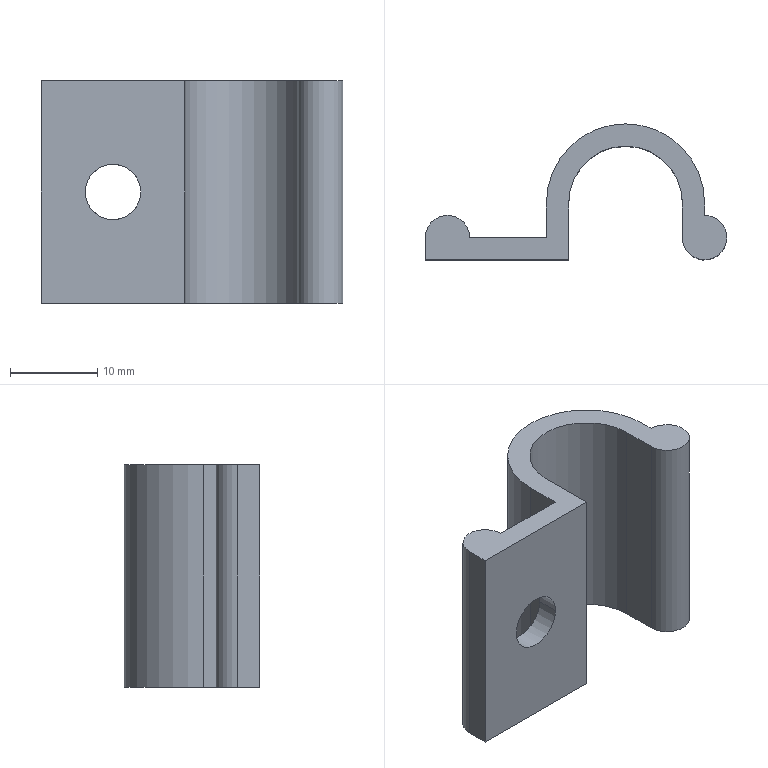Part | STEP file | tubing_clipV11_6.01 - 12.70mm Dia | 1 solid | 15 faces | box 34.48 x 15.54 x 25.4 mm | volume 3707 mm3 | plane 9 | cylinder 6 | commonest cylinder face diameters 5.08 x2 6.35 x2 13 x1 18.08 x1
STEP:
#1=CARTESIAN_POINT('',(0.,0.,0.));
#2=DIRECTION('',(0.,0.,1.));
#3=DIRECTION('',(1.,0.,0.));
#4=AXIS2_PLACEMENT_3D('',#1,#2,#3);
#5=CARTESIAN_POINT('',(-17.82,-3.96,-0.5884));
#6=VERTEX_POINT('',#5);
#7=CARTESIAN_POINT('',(-11.525,-3.96,0.));
#8=VERTEX_POINT('',#7);
#9=CARTESIAN_POINT('',(-14.7,-3.96,0.));
#10=DIRECTION('',(0.,-1.,0.));
#11=DIRECTION('',(1.,0.,0.));
#12=AXIS2_PLACEMENT_3D('',#9,#10,#11);
#13=CIRCLE('',#12,3.175);
#14=CARTESIAN_POINT('',(-14.7,9.04,0.));
#15=DIRECTION('',(0.,-1.,0.));
#16=DIRECTION('',(1.,0.,0.));
#17=AXIS2_PLACEMENT_3D('',#14,#15,#16);
#18=CYLINDRICAL_SURFACE('',#17,3.175);
#19=CARTESIAN_POINT('',(0.,13.));
#20=DIRECTION('',(1.,0.));
#21=VECTOR('',#20,1.);
#22=LINE('',#19,#21);
#23=(GEOMETRIC_REPRESENTATION_CONTEXT(2)PARAMETRIC_REPRESENTATION_CONTEXT()REPRESENTATION_CONTEXT('',''));
#24=DEFINITIONAL_REPRESENTATION('',(#22),#23);
#25=PCURVE('',#18,#24);
#26=CARTESIAN_POINT('',(-17.82,-3.96,12.7));
#27=DIRECTION('',(0.,-1.,0.));
#28=DIRECTION('',(1.,0.,0.));
#29=AXIS2_PLACEMENT_3D('',#26,#27,#28);
#30=PLANE('',#29);
#31=CARTESIAN_POINT('',(3.12,-12.7));
#32=DIRECTION('',(1.,0.));
#33=AXIS2_PLACEMENT_2D('',#31,#32);
#34=CIRCLE('',#33,3.175);
#35=(GEOMETRIC_REPRESENTATION_CONTEXT(2)PARAMETRIC_REPRESENTATION_CONTEXT()REPRESENTATION_CONTEXT('',''));
#36=DEFINITIONAL_REPRESENTATION('',(#34),#35);
#37=PCURVE('',#30,#36);
#38=SURFACE_CURVE('',#13,(#25,#37),.PCURVE_S1.);
#39=EDGE_CURVE('',#6,#8,#38,.T.);
#40=ORIENTED_EDGE('',*,*,#39,.T.);
#41=CARTESIAN_POINT('',(-11.525,-6.5,0.));
#42=VERTEX_POINT('',#41);
#43=CARTESIAN_POINT('',(-11.525,9.04,0.));
#44=DIRECTION('',(0.,-1.,0.));
#45=VECTOR('',#44,1.);
#46=LINE('',#43,#45);
#47=CARTESIAN_POINT('',(6.283,0.));
#48=DIRECTION('',(0.,1.));
#49=VECTOR('',#48,1.);
#50=LINE('',#47,#49);
#51=(GEOMETRIC_REPRESENTATION_CONTEXT(2)PARAMETRIC_REPRESENTATION_CONTEXT()REPRESENTATION_CONTEXT('',''));
#52=DEFINITIONAL_REPRESENTATION('',(#50),#51);
#53=PCURVE('',#18,#52);
#54=CARTESIAN_POINT('',(-14.7,9.04,0.));
#55=DIRECTION('',(0.,-1.,0.));
#56=DIRECTION('',(1.,0.,0.));
#57=AXIS2_PLACEMENT_3D('',#54,#55,#56);
#58=CYLINDRICAL_SURFACE('',#57,3.175);
#59=CARTESIAN_POINT('',(0.,0.));
#60=DIRECTION('',(0.,1.));
#61=VECTOR('',#60,1.);
#62=LINE('',#59,#61);
#63=(GEOMETRIC_REPRESENTATION_CONTEXT(2)PARAMETRIC_REPRESENTATION_CONTEXT()REPRESENTATION_CONTEXT('',''));
#64=DEFINITIONAL_REPRESENTATION('',(#62),#63);
#65=PCURVE('',#58,#64);
#66=SURFACE_CURVE('',#46,(#53,#65),.PCURVE_S1.);
#67=EDGE_CURVE('',#8,#42,#66,.T.);
#68=ORIENTED_EDGE('',*,*,#67,.T.);
#69=CARTESIAN_POINT('',(-17.875,-6.5,0.));
#70=VERTEX_POINT('',#69);
#71=CARTESIAN_POINT('',(-14.7,-6.5,0.));
#72=DIRECTION('',(0.,-1.,0.));
#73=DIRECTION('',(1.,0.,0.));
#74=AXIS2_PLACEMENT_3D('',#71,#72,#73);
#75=CIRCLE('',#74,3.175);
#76=CARTESIAN_POINT('',(0.,15.54));
#77=DIRECTION('',(1.,0.));
#78=VECTOR('',#77,1.);
#79=LINE('',#76,#78);
#80=(GEOMETRIC_REPRESENTATION_CONTEXT(2)PARAMETRIC_REPRESENTATION_CONTEXT()REPRESENTATION_CONTEXT('',''));
#81=DEFINITIONAL_REPRESENTATION('',(#79),#80);
#82=PCURVE('',#18,#81);
#83=CARTESIAN_POINT('',(-6.5,-6.5,12.7));
#84=DIRECTION('',(0.,1.,0.));
#85=DIRECTION('',(-1.,0.,0.));
#86=AXIS2_PLACEMENT_3D('',#83,#84,#85);
#87=PLANE('',#86);
#88=CARTESIAN_POINT('',(5.025,-12.7));
#89=CARTESIAN_POINT('',(5.025,-7.201));
#90=CARTESIAN_POINT('',(9.787,-9.95));
#91=CARTESIAN_POINT('',(14.55,-12.7));
#92=CARTESIAN_POINT('',(9.787,-15.45));
#93=CARTESIAN_POINT('',(5.025,-18.199));
#94=CARTESIAN_POINT('',(5.025,-12.7));
#95=(BOUNDED_CURVE()B_SPLINE_CURVE(2,(#88,#89,#90,#91,#92,#93,#94),.UNSPECIFIED.,.T.,.F.)B_SPLINE_CURVE_WITH_KNOTS((1,2,2,2,2,1),(-2.094,0.,2.094,4.189,6.283,8.378),.UNSPECIFIED.)CURVE()GEOMETRIC_REPRESENTATION_ITEM()RATIONAL_B_SPLINE_CURVE((1.,0.5,1.,0.5,1.,0.5,1.))REPRESENTATION_ITEM(''));
#96=(GEOMETRIC_REPRESENTATION_CONTEXT(2)PARAMETRIC_REPRESENTATION_CONTEXT()REPRESENTATION_CONTEXT('',''));
#97=DEFINITIONAL_REPRESENTATION('',(#95),#96);
#98=PCURVE('',#87,#97);
#99=SURFACE_CURVE('',#75,(#82,#98),.PCURVE_S1.);
#100=EDGE_CURVE('',#70,#42,#99,.T.);
#101=ORIENTED_EDGE('',*,*,#100,.F.);
#102=CARTESIAN_POINT('',(-17.875,-3.434,0.));
#103=VERTEX_POINT('',#102);
#104=CARTESIAN_POINT('',(-17.875,9.04,0.));
#105=DIRECTION('',(0.,-1.,0.));
#106=VECTOR('',#105,1.);
#107=LINE('',#104,#106);
#108=CARTESIAN_POINT('',(3.142,0.));
#109=DIRECTION('',(0.,1.));
#110=VECTOR('',#109,1.);
#111=LINE('',#108,#110);
#112=(GEOMETRIC_REPRESENTATION_CONTEXT(2)PARAMETRIC_REPRESENTATION_CONTEXT()REPRESENTATION_CONTEXT('',''));
#113=DEFINITIONAL_REPRESENTATION('',(#111),#112);
#114=PCURVE('',#18,#113);
#115=CARTESIAN_POINT('',(3.142,0.));
#116=DIRECTION('',(0.,1.));
#117=VECTOR('',#116,1.);
#118=LINE('',#115,#117);
#119=(GEOMETRIC_REPRESENTATION_CONTEXT(2)PARAMETRIC_REPRESENTATION_CONTEXT()REPRESENTATION_CONTEXT('',''));
#120=DEFINITIONAL_REPRESENTATION('',(#118),#119);
#121=PCURVE('',#58,#120);
#122=SURFACE_CURVE('',#107,(#114,#121),.PCURVE_S1.);
#123=EDGE_CURVE('',#103,#70,#122,.T.);
#124=ORIENTED_EDGE('',*,*,#123,.F.);
#125=CARTESIAN_POINT('',(-17.875,-3.434,0.));
#126=CARTESIAN_POINT('',(-17.875,-3.434,-0.1473));
#127=CARTESIAN_POINT('',(-17.864,-3.482,-0.2926));
#128=CARTESIAN_POINT('',(-17.835,-3.671,-0.5171));
#129=CARTESIAN_POINT('',(-17.82,-3.812,-0.5884));
#130=CARTESIAN_POINT('',(-17.82,-3.96,-0.5884));
#131=B_SPLINE_CURVE_WITH_KNOTS('',3,(#125,#126,#127,#128,#129,#130),.UNSPECIFIED.,.F.,.F.,(4,2,4),(0.0008744,0.001312,0.00175),.UNSPECIFIED.);
#132=CARTESIAN_POINT('',(3.142,12.474));
#133=CARTESIAN_POINT('',(3.146,12.474));
#134=CARTESIAN_POINT('',(3.154,12.475));
#135=CARTESIAN_POINT('',(3.167,12.479));
#136=CARTESIAN_POINT('',(3.179,12.485));
#137=CARTESIAN_POINT('',(3.192,12.493));
#138=CARTESIAN_POINT('',(3.204,12.503));
#139=CARTESIAN_POINT('',(3.215,12.516));
#140=CARTESIAN_POINT('',(3.227,12.532));
#141=CARTESIAN_POINT('',(3.238,12.549));
#142=CARTESIAN_POINT('',(3.249,12.569));
#143=CARTESIAN_POINT('',(3.26,12.592));
#144=CARTESIAN_POINT('',(3.27,12.616));
#145=CARTESIAN_POINT('',(3.279,12.643));
#146=CARTESIAN_POINT('',(3.288,12.672));
#147=CARTESIAN_POINT('',(3.296,12.703));
#148=CARTESIAN_POINT('',(3.303,12.736));
#149=CARTESIAN_POINT('',(3.309,12.77));
#150=CARTESIAN_POINT('',(3.315,12.806));
#151=CARTESIAN_POINT('',(3.32,12.843));
#152=CARTESIAN_POINT('',(3.323,12.881));
#153=CARTESIAN_POINT('',(3.326,12.92));
#154=CARTESIAN_POINT('',(3.328,12.96));
#155=CARTESIAN_POINT('',(3.328,12.987));
#156=CARTESIAN_POINT('',(3.328,13.));
#157=B_SPLINE_CURVE_WITH_KNOTS('',3,(#132,#133,#134,#135,#136,#137,#138,#139,#140,#141,#142,#143,#144,#145,#146,#147,#148,#149,#150,#151,#152,#153,#154,#155,#156),.UNSPECIFIED.,.F.,.F.,(4,1,1,1,1,1,1,1,1,1,1,1,1,1,1,1,1,1,1,1,1,1,4),(0.0008744,0.0009142,0.000954,0.0009938,0.001034,0.001073,0.001113,0.001153,0.001193,0.001233,0.001272,0.001312,0.001352,0.001392,0.001432,0.001471,0.001511,0.001551,0.001591,0.00163,0.00167,0.00171,0.00175),.QUASI_UNIFORM_KNOTS.);
#158=(GEOMETRIC_REPRESENTATION_CONTEXT(2)PARAMETRIC_REPRESENTATION_CONTEXT()REPRESENTATION_CONTEXT('',''));
#159=DEFINITIONAL_REPRESENTATION('',(#157),#158);
#160=PCURVE('',#18,#159);
#161=CARTESIAN_POINT('',(-20.36,-3.96,12.7));
#162=DIRECTION('',(0.,0.,-1.));
#163=DIRECTION('',(-1.,0.,0.));
#164=AXIS2_PLACEMENT_3D('',#161,#162,#163);
#165=CYLINDRICAL_SURFACE('',#164,2.54);
#166=CARTESIAN_POINT('',(2.933,12.7));
#167=CARTESIAN_POINT('',(2.933,12.713));
#168=CARTESIAN_POINT('',(2.933,12.74));
#169=CARTESIAN_POINT('',(2.935,12.78));
#170=CARTESIAN_POINT('',(2.937,12.82));
#171=CARTESIAN_POINT('',(2.941,12.859));
#172=CARTESIAN_POINT('',(2.945,12.897));
#173=CARTESIAN_POINT('',(2.95,12.934));
#174=CARTESIAN_POINT('',(2.956,12.971));
#175=CARTESIAN_POINT('',(2.963,13.006));
#176=CARTESIAN_POINT('',(2.971,13.041));
#177=CARTESIAN_POINT('',(2.98,13.074));
#178=CARTESIAN_POINT('',(2.99,13.105));
#179=CARTESIAN_POINT('',(3.001,13.135));
#180=CARTESIAN_POINT('',(3.012,13.162));
#181=CARTESIAN_POINT('',(3.024,13.187));
#182=CARTESIAN_POINT('',(3.037,13.21));
#183=CARTESIAN_POINT('',(3.051,13.23));
#184=CARTESIAN_POINT('',(3.065,13.248));
#185=CARTESIAN_POINT('',(3.08,13.262));
#186=CARTESIAN_POINT('',(3.095,13.274));
#187=CARTESIAN_POINT('',(3.11,13.282));
#188=CARTESIAN_POINT('',(3.126,13.287));
#189=CARTESIAN_POINT('',(3.136,13.288));
#190=CARTESIAN_POINT('',(3.142,13.288));
#191=B_SPLINE_CURVE_WITH_KNOTS('',3,(#166,#167,#168,#169,#170,#171,#172,#173,#174,#175,#176,#177,#178,#179,#180,#181,#182,#183,#184,#185,#186,#187,#188,#189,#190),.UNSPECIFIED.,.F.,.F.,(4,1,1,1,1,1,1,1,1,1,1,1,1,1,1,1,1,1,1,1,1,1,4),(0.0008744,0.0009142,0.000954,0.0009938,0.001034,0.001073,0.001113,0.001153,0.001193,0.001233,0.001272,0.001312,0.001352,0.001392,0.001432,0.001471,0.001511,0.001551,0.001591,0.00163,0.00167,0.00171,0.00175),.QUASI_UNIFORM_KNOTS.);
#192=(GEOMETRIC_REPRESENTATION_CONTEXT(2)PARAMETRIC_REPRESENTATION_CONTEXT()REPRESENTATION_CONTEXT('',''));
#193=DEFINITIONAL_REPRESENTATION('',(#191),#192);
#194=PCURVE('',#165,#193);
#195=SURFACE_CURVE('',#131,(#160,#194),.PCURVE_S1.);
#196=EDGE_CURVE('',#103,#6,#195,.T.);
#197=ORIENTED_EDGE('',*,*,#196,.T.);
#198=EDGE_LOOP('',(#40,#68,#101,#124,#197));
#199=FACE_BOUND('',#198,.F.);
#200=ADVANCED_FACE('',(#199),#18,.F.);
#201=CARTESIAN_POINT('',(-14.7,-6.5,0.));
#202=DIRECTION('',(0.,-1.,0.));
#203=DIRECTION('',(1.,0.,0.));
#204=AXIS2_PLACEMENT_3D('',#201,#202,#203);
#205=CIRCLE('',#204,3.175);
#206=CARTESIAN_POINT('',(5.025,-12.7));
#207=CARTESIAN_POINT('',(5.025,-7.201));
#208=CARTESIAN_POINT('',(9.787,-9.95));
#209=CARTESIAN_POINT('',(14.55,-12.7));
#210=CARTESIAN_POINT('',(9.787,-15.45));
#211=CARTESIAN_POINT('',(5.025,-18.199));
#212=CARTESIAN_POINT('',(5.025,-12.7));
#213=(BOUNDED_CURVE()B_SPLINE_CURVE(2,(#206,#207,#208,#209,#210,#211,#212),.UNSPECIFIED.,.T.,.F.)B_SPLINE_CURVE_WITH_KNOTS((1,2,2,2,2,1),(-2.094,0.,2.094,4.189,6.283,8.378),.UNSPECIFIED.)CURVE()GEOMETRIC_REPRESENTATION_ITEM()RATIONAL_B_SPLINE_CURVE((1.,0.5,1.,0.5,1.,0.5,1.))REPRESENTATION_ITEM(''));
#214=(GEOMETRIC_REPRESENTATION_CONTEXT(2)PARAMETRIC_REPRESENTATION_CONTEXT()REPRESENTATION_CONTEXT('',''));
#215=DEFINITIONAL_REPRESENTATION('',(#213),#214);
#216=PCURVE('',#87,#215);
#217=CARTESIAN_POINT('',(0.,15.54));
#218=DIRECTION('',(1.,0.));
#219=VECTOR('',#218,1.);
#220=LINE('',#217,#219);
#221=(GEOMETRIC_REPRESENTATION_CONTEXT(2)PARAMETRIC_REPRESENTATION_CONTEXT()REPRESENTATION_CONTEXT('',''));
#222=DEFINITIONAL_REPRESENTATION('',(#220),#221);
#223=PCURVE('',#58,#222);
#224=SURFACE_CURVE('',#205,(#216,#223),.PCURVE_S1.);
#225=EDGE_CURVE('',#42,#70,#224,.T.);
#226=ORIENTED_EDGE('',*,*,#225,.F.);
#227=ORIENTED_EDGE('',*,*,#100,.F.);
#228=EDGE_LOOP('',(#226,#227));
#229=FACE_BOUND('',#228,.T.);
#230=CARTESIAN_POINT('',(-22.9,-6.5,-12.7));
#231=VERTEX_POINT('',#230);
#232=CARTESIAN_POINT('',(-6.5,-6.5,-12.7));
#233=VERTEX_POINT('',#232);
#234=CARTESIAN_POINT('',(-6.5,-6.5,-12.7));
#235=DIRECTION('',(1.,0.,0.));
#236=VECTOR('',#235,1.);
#237=LINE('',#234,#236);
#238=CARTESIAN_POINT('',(0.,-25.4));
#239=DIRECTION('',(-1.,0.));
#240=VECTOR('',#239,1.);
#241=LINE('',#238,#240);
#242=(GEOMETRIC_REPRESENTATION_CONTEXT(2)PARAMETRIC_REPRESENTATION_CONTEXT()REPRESENTATION_CONTEXT('',''));
#243=DEFINITIONAL_REPRESENTATION('',(#241),#242);
#244=PCURVE('',#87,#243);
#245=CARTESIAN_POINT('',(-20.36,-3.96,-12.7));
#246=DIRECTION('',(0.,0.,1.));
#247=DIRECTION('',(1.,0.,0.));
#248=AXIS2_PLACEMENT_3D('',#245,#246,#247);
#249=PLANE('',#248);
#250=CARTESIAN_POINT('',(13.86,-2.54));
#251=DIRECTION('',(1.,0.));
#252=VECTOR('',#251,1.);
#253=LINE('',#250,#252);
#254=(GEOMETRIC_REPRESENTATION_CONTEXT(2)PARAMETRIC_REPRESENTATION_CONTEXT()REPRESENTATION_CONTEXT('',''));
#255=DEFINITIONAL_REPRESENTATION('',(#253),#254);
#256=PCURVE('',#249,#255);
#257=SURFACE_CURVE('',#237,(#244,#256),.PCURVE_S1.);
#258=EDGE_CURVE('',#231,#233,#257,.T.);
#259=ORIENTED_EDGE('',*,*,#258,.T.);
#260=CARTESIAN_POINT('',(-6.5,-6.5,12.7));
#261=VERTEX_POINT('',#260);
#262=CARTESIAN_POINT('',(-6.5,-6.5,12.7));
#263=DIRECTION('',(0.,0.,-1.));
#264=VECTOR('',#263,1.);
#265=LINE('',#262,#264);
#266=CARTESIAN_POINT('',(0.,0.));
#267=DIRECTION('',(0.,-1.));
#268=VECTOR('',#267,1.);
#269=LINE('',#266,#268);
#270=(GEOMETRIC_REPRESENTATION_CONTEXT(2)PARAMETRIC_REPRESENTATION_CONTEXT()REPRESENTATION_CONTEXT('',''));
#271=DEFINITIONAL_REPRESENTATION('',(#269),#270);
#272=PCURVE('',#87,#271);
#273=CARTESIAN_POINT('',(-6.5,0.,12.7));
#274=DIRECTION('',(-1.,0.,0.));
#275=DIRECTION('',(0.,-1.,0.));
#276=AXIS2_PLACEMENT_3D('',#273,#274,#275);
#277=PLANE('',#276);
#278=CARTESIAN_POINT('',(6.5,0.));
#279=DIRECTION('',(0.,-1.));
#280=VECTOR('',#279,1.);
#281=LINE('',#278,#280);
#282=(GEOMETRIC_REPRESENTATION_CONTEXT(2)PARAMETRIC_REPRESENTATION_CONTEXT()REPRESENTATION_CONTEXT('',''));
#283=DEFINITIONAL_REPRESENTATION('',(#281),#282);
#284=PCURVE('',#277,#283);
#285=SURFACE_CURVE('',#265,(#272,#284),.PCURVE_S1.);
#286=EDGE_CURVE('',#261,#233,#285,.T.);
#287=ORIENTED_EDGE('',*,*,#286,.F.);
#288=CARTESIAN_POINT('',(-22.9,-6.5,12.7));
#289=VERTEX_POINT('',#288);
#290=CARTESIAN_POINT('',(-6.5,-6.5,12.7));
#291=DIRECTION('',(1.,0.,0.));
#292=VECTOR('',#291,1.);
#293=LINE('',#290,#292);
#294=CARTESIAN_POINT('',(0.,0.));
#295=DIRECTION('',(-1.,0.));
#296=VECTOR('',#295,1.);
#297=LINE('',#294,#296);
#298=(GEOMETRIC_REPRESENTATION_CONTEXT(2)PARAMETRIC_REPRESENTATION_CONTEXT()REPRESENTATION_CONTEXT('',''));
#299=DEFINITIONAL_REPRESENTATION('',(#297),#298);
#300=PCURVE('',#87,#299);
#301=CARTESIAN_POINT('',(-20.36,-3.96,12.7));
#302=DIRECTION('',(0.,0.,1.));
#303=DIRECTION('',(1.,0.,0.));
#304=AXIS2_PLACEMENT_3D('',#301,#302,#303);
#305=PLANE('',#304);
#306=CARTESIAN_POINT('',(13.86,-2.54));
#307=DIRECTION('',(1.,0.));
#308=VECTOR('',#307,1.);
#309=LINE('',#306,#308);
#310=(GEOMETRIC_REPRESENTATION_CONTEXT(2)PARAMETRIC_REPRESENTATION_CONTEXT()REPRESENTATION_CONTEXT('',''));
#311=DEFINITIONAL_REPRESENTATION('',(#309),#310);
#312=PCURVE('',#305,#311);
#313=SURFACE_CURVE('',#293,(#300,#312),.PCURVE_S1.);
#314=EDGE_CURVE('',#289,#261,#313,.T.);
#315=ORIENTED_EDGE('',*,*,#314,.F.);
#316=CARTESIAN_POINT('',(-22.9,-6.5,12.7));
#317=DIRECTION('',(0.,0.,-1.));
#318=VECTOR('',#317,1.);
#319=LINE('',#316,#318);
#320=CARTESIAN_POINT('',(16.4,0.));
#321=DIRECTION('',(0.,-1.));
#322=VECTOR('',#321,1.);
#323=LINE('',#320,#322);
#324=(GEOMETRIC_REPRESENTATION_CONTEXT(2)PARAMETRIC_REPRESENTATION_CONTEXT()REPRESENTATION_CONTEXT('',''));
#325=DEFINITIONAL_REPRESENTATION('',(#323),#324);
#326=PCURVE('',#87,#325);
#327=CARTESIAN_POINT('',(-22.9,-6.5,12.7));
#328=DIRECTION('',(1.,0.,0.));
#329=DIRECTION('',(0.,0.,-1.));
#330=AXIS2_PLACEMENT_3D('',#327,#328,#329);
#331=PLANE('',#330);
#332=CARTESIAN_POINT('',(0.,0.));
#333=DIRECTION('',(1.,0.));
#334=VECTOR('',#333,1.);
#335=LINE('',#332,#334);
#336=(GEOMETRIC_REPRESENTATION_CONTEXT(2)PARAMETRIC_REPRESENTATION_CONTEXT()REPRESENTATION_CONTEXT('',''));
#337=DEFINITIONAL_REPRESENTATION('',(#335),#336);
#338=PCURVE('',#331,#337);
#339=SURFACE_CURVE('',#319,(#326,#338),.PCURVE_S1.);
#340=EDGE_CURVE('',#289,#231,#339,.T.);
#341=ORIENTED_EDGE('',*,*,#340,.T.);
#342=EDGE_LOOP('',(#259,#287,#315,#341));
#343=FACE_BOUND('',#342,.T.);
#344=ADVANCED_FACE('',(#229,#343),#87,.F.);
#345=CARTESIAN_POINT('',(-6.5,0.,-12.7));
#346=VERTEX_POINT('',#345);
#347=CARTESIAN_POINT('',(-6.5,0.,-12.7));
#348=DIRECTION('',(0.,1.,0.));
#349=VECTOR('',#348,1.);
#350=LINE('',#347,#349);
#351=CARTESIAN_POINT('',(0.,-25.4));
#352=DIRECTION('',(-1.,0.));
#353=VECTOR('',#352,1.);
#354=LINE('',#351,#353);
#355=(GEOMETRIC_REPRESENTATION_CONTEXT(2)PARAMETRIC_REPRESENTATION_CONTEXT()REPRESENTATION_CONTEXT('',''));
#356=DEFINITIONAL_REPRESENTATION('',(#354),#355);
#357=PCURVE('',#277,#356);
#358=CARTESIAN_POINT('',(13.86,3.96));
#359=DIRECTION('',(0.,1.));
#360=VECTOR('',#359,1.);
#361=LINE('',#358,#360);
#362=(GEOMETRIC_REPRESENTATION_CONTEXT(2)PARAMETRIC_REPRESENTATION_CONTEXT()REPRESENTATION_CONTEXT('',''));
#363=DEFINITIONAL_REPRESENTATION('',(#361),#362);
#364=PCURVE('',#249,#363);
#365=SURFACE_CURVE('',#350,(#357,#364),.PCURVE_S1.);
#366=EDGE_CURVE('',#233,#346,#365,.T.);
#367=ORIENTED_EDGE('',*,*,#366,.T.);
#368=CARTESIAN_POINT('',(-6.5,0.,12.7));
#369=VERTEX_POINT('',#368);
#370=CARTESIAN_POINT('',(-6.5,0.,12.7));
#371=DIRECTION('',(0.,0.,-1.));
#372=VECTOR('',#371,1.);
#373=LINE('',#370,#372);
#374=CARTESIAN_POINT('',(0.,0.));
#375=DIRECTION('',(0.,-1.));
#376=VECTOR('',#375,1.);
#377=LINE('',#374,#376);
#378=(GEOMETRIC_REPRESENTATION_CONTEXT(2)PARAMETRIC_REPRESENTATION_CONTEXT()REPRESENTATION_CONTEXT('',''));
#379=DEFINITIONAL_REPRESENTATION('',(#377),#378);
#380=PCURVE('',#277,#379);
#381=CARTESIAN_POINT('',(0.,0.,12.7));
#382=DIRECTION('',(0.,0.,-1.));
#383=DIRECTION('',(-1.,0.,0.));
#384=AXIS2_PLACEMENT_3D('',#381,#382,#383);
#385=CYLINDRICAL_SURFACE('',#384,6.5);
#386=CARTESIAN_POINT('',(0.,0.));
#387=DIRECTION('',(0.,1.));
#388=VECTOR('',#387,1.);
#389=LINE('',#386,#388);
#390=(GEOMETRIC_REPRESENTATION_CONTEXT(2)PARAMETRIC_REPRESENTATION_CONTEXT()REPRESENTATION_CONTEXT('',''));
#391=DEFINITIONAL_REPRESENTATION('',(#389),#390);
#392=PCURVE('',#385,#391);
#393=SURFACE_CURVE('',#373,(#380,#392),.PCURVE_S1.);
#394=EDGE_CURVE('',#369,#346,#393,.T.);
#395=ORIENTED_EDGE('',*,*,#394,.F.);
#396=CARTESIAN_POINT('',(-6.5,0.,12.7));
#397=DIRECTION('',(0.,1.,0.));
#398=VECTOR('',#397,1.);
#399=LINE('',#396,#398);
#400=CARTESIAN_POINT('',(0.,0.));
#401=DIRECTION('',(-1.,0.));
#402=VECTOR('',#401,1.);
#403=LINE('',#400,#402);
#404=(GEOMETRIC_REPRESENTATION_CONTEXT(2)PARAMETRIC_REPRESENTATION_CONTEXT()REPRESENTATION_CONTEXT('',''));
#405=DEFINITIONAL_REPRESENTATION('',(#403),#404);
#406=PCURVE('',#277,#405);
#407=CARTESIAN_POINT('',(13.86,3.96));
#408=DIRECTION('',(0.,1.));
#409=VECTOR('',#408,1.);
#410=LINE('',#407,#409);
#411=(GEOMETRIC_REPRESENTATION_CONTEXT(2)PARAMETRIC_REPRESENTATION_CONTEXT()REPRESENTATION_CONTEXT('',''));
#412=DEFINITIONAL_REPRESENTATION('',(#410),#411);
#413=PCURVE('',#305,#412);
#414=SURFACE_CURVE('',#399,(#406,#413),.PCURVE_S1.);
#415=EDGE_CURVE('',#261,#369,#414,.T.);
#416=ORIENTED_EDGE('',*,*,#415,.F.);
#417=ORIENTED_EDGE('',*,*,#286,.T.);
#418=EDGE_LOOP('',(#367,#395,#416,#417));
#419=FACE_BOUND('',#418,.T.);
#420=ADVANCED_FACE('',(#419),#277,.F.);
#421=ORIENTED_EDGE('',*,*,#394,.F.);
#422=CARTESIAN_POINT('',(6.5,0.,12.7));
#423=VERTEX_POINT('',#422);
#424=CARTESIAN_POINT('',(0.,0.,12.7));
#425=DIRECTION('',(0.,0.,-1.));
#426=DIRECTION('',(1.,0.,0.));
#427=AXIS2_PLACEMENT_3D('',#424,#425,#426);
#428=CIRCLE('',#427,6.5);
#429=CARTESIAN_POINT('',(-3.142,0.));
#430=DIRECTION('',(1.,0.));
#431=VECTOR('',#430,1.);
#432=LINE('',#429,#431);
#433=(GEOMETRIC_REPRESENTATION_CONTEXT(2)PARAMETRIC_REPRESENTATION_CONTEXT()REPRESENTATION_CONTEXT('',''));
#434=DEFINITIONAL_REPRESENTATION('',(#432),#433);
#435=PCURVE('',#385,#434);
#436=CARTESIAN_POINT('',(26.86,3.96));
#437=CARTESIAN_POINT('',(26.86,-7.298));
#438=CARTESIAN_POINT('',(17.11,-1.669));
#439=CARTESIAN_POINT('',(7.36,3.96));
#440=CARTESIAN_POINT('',(17.11,9.589));
#441=CARTESIAN_POINT('',(26.86,15.218));
#442=CARTESIAN_POINT('',(26.86,3.96));
#443=(BOUNDED_CURVE()B_SPLINE_CURVE(2,(#436,#437,#438,#439,#440,#441,#442),.UNSPECIFIED.,.T.,.F.)B_SPLINE_CURVE_WITH_KNOTS((1,2,2,2,2,1),(-2.094,0.,2.094,4.189,6.283,8.378),.UNSPECIFIED.)CURVE()GEOMETRIC_REPRESENTATION_ITEM()RATIONAL_B_SPLINE_CURVE((1.,0.5,1.,0.5,1.,0.5,1.))REPRESENTATION_ITEM(''));
#444=(GEOMETRIC_REPRESENTATION_CONTEXT(2)PARAMETRIC_REPRESENTATION_CONTEXT()REPRESENTATION_CONTEXT('',''));
#445=DEFINITIONAL_REPRESENTATION('',(#443),#444);
#446=PCURVE('',#305,#445);
#447=SURFACE_CURVE('',#428,(#435,#446),.PCURVE_S1.);
#448=EDGE_CURVE('',#369,#423,#447,.T.);
#449=ORIENTED_EDGE('',*,*,#448,.T.);
#450=CARTESIAN_POINT('',(6.5,0.,-12.7));
#451=VERTEX_POINT('',#450);
#452=CARTESIAN_POINT('',(6.5,0.,12.7));
#453=DIRECTION('',(0.,0.,-1.));
#454=VECTOR('',#453,1.);
#455=LINE('',#452,#454);
#456=CARTESIAN_POINT('',(3.142,0.));
#457=DIRECTION('',(0.,1.));
#458=VECTOR('',#457,1.);
#459=LINE('',#456,#458);
#460=(GEOMETRIC_REPRESENTATION_CONTEXT(2)PARAMETRIC_REPRESENTATION_CONTEXT()REPRESENTATION_CONTEXT('',''));
#461=DEFINITIONAL_REPRESENTATION('',(#459),#460);
#462=PCURVE('',#385,#461);
#463=CARTESIAN_POINT('',(6.5,0.,12.7));
#464=DIRECTION('',(1.,0.,0.));
#465=DIRECTION('',(0.,1.,0.));
#466=AXIS2_PLACEMENT_3D('',#463,#464,#465);
#467=PLANE('',#466);
#468=CARTESIAN_POINT('',(0.,0.));
#469=DIRECTION('',(0.,-1.));
#470=VECTOR('',#469,1.);
#471=LINE('',#468,#470);
#472=(GEOMETRIC_REPRESENTATION_CONTEXT(2)PARAMETRIC_REPRESENTATION_CONTEXT()REPRESENTATION_CONTEXT('',''));
#473=DEFINITIONAL_REPRESENTATION('',(#471),#472);
#474=PCURVE('',#467,#473);
#475=SURFACE_CURVE('',#455,(#462,#474),.PCURVE_S1.);
#476=EDGE_CURVE('',#423,#451,#475,.T.);
#477=ORIENTED_EDGE('',*,*,#476,.T.);
#478=CARTESIAN_POINT('',(0.,0.,-12.7));
#479=DIRECTION('',(0.,0.,-1.));
#480=DIRECTION('',(1.,0.,0.));
#481=AXIS2_PLACEMENT_3D('',#478,#479,#480);
#482=CIRCLE('',#481,6.5);
#483=CARTESIAN_POINT('',(-3.142,25.4));
#484=DIRECTION('',(1.,0.));
#485=VECTOR('',#484,1.);
#486=LINE('',#483,#485);
#487=(GEOMETRIC_REPRESENTATION_CONTEXT(2)PARAMETRIC_REPRESENTATION_CONTEXT()REPRESENTATION_CONTEXT('',''));
#488=DEFINITIONAL_REPRESENTATION('',(#486),#487);
#489=PCURVE('',#385,#488);
#490=CARTESIAN_POINT('',(26.86,3.96));
#491=CARTESIAN_POINT('',(26.86,-7.298));
#492=CARTESIAN_POINT('',(17.11,-1.669));
#493=CARTESIAN_POINT('',(7.36,3.96));
#494=CARTESIAN_POINT('',(17.11,9.589));
#495=CARTESIAN_POINT('',(26.86,15.218));
#496=CARTESIAN_POINT('',(26.86,3.96));
#497=(BOUNDED_CURVE()B_SPLINE_CURVE(2,(#490,#491,#492,#493,#494,#495,#496),.UNSPECIFIED.,.T.,.F.)B_SPLINE_CURVE_WITH_KNOTS((1,2,2,2,2,1),(-2.094,0.,2.094,4.189,6.283,8.378),.UNSPECIFIED.)CURVE()GEOMETRIC_REPRESENTATION_ITEM()RATIONAL_B_SPLINE_CURVE((1.,0.5,1.,0.5,1.,0.5,1.))REPRESENTATION_ITEM(''));
#498=(GEOMETRIC_REPRESENTATION_CONTEXT(2)PARAMETRIC_REPRESENTATION_CONTEXT()REPRESENTATION_CONTEXT('',''));
#499=DEFINITIONAL_REPRESENTATION('',(#497),#498);
#500=PCURVE('',#249,#499);
#501=SURFACE_CURVE('',#482,(#489,#500),.PCURVE_S1.);
#502=EDGE_CURVE('',#346,#451,#501,.T.);
#503=ORIENTED_EDGE('',*,*,#502,.F.);
#504=EDGE_LOOP('',(#421,#449,#477,#503));
#505=FACE_BOUND('',#504,.F.);
#506=ADVANCED_FACE('',(#505),#385,.F.);
#507=CARTESIAN_POINT('',(6.5,-3.96,-12.7));
#508=VERTEX_POINT('',#507);
#509=CARTESIAN_POINT('',(6.5,0.,-12.7));
#510=DIRECTION('',(0.,-1.,0.));
#511=VECTOR('',#510,1.);
#512=LINE('',#509,#511);
#513=CARTESIAN_POINT('',(0.,-25.4));
#514=DIRECTION('',(-1.,0.));
#515=VECTOR('',#514,1.);
#516=LINE('',#513,#515);
#517=(GEOMETRIC_REPRESENTATION_CONTEXT(2)PARAMETRIC_REPRESENTATION_CONTEXT()REPRESENTATION_CONTEXT('',''));
#518=DEFINITIONAL_REPRESENTATION('',(#516),#517);
#519=PCURVE('',#467,#518);
#520=CARTESIAN_POINT('',(26.86,3.96));
#521=DIRECTION('',(0.,-1.));
#522=VECTOR('',#521,1.);
#523=LINE('',#520,#522);
#524=(GEOMETRIC_REPRESENTATION_CONTEXT(2)PARAMETRIC_REPRESENTATION_CONTEXT()REPRESENTATION_CONTEXT('',''));
#525=DEFINITIONAL_REPRESENTATION('',(#523),#524);
#526=PCURVE('',#249,#525);
#527=SURFACE_CURVE('',#512,(#519,#526),.PCURVE_S1.);
#528=EDGE_CURVE('',#451,#508,#527,.T.);
#529=ORIENTED_EDGE('',*,*,#528,.T.);
#530=CARTESIAN_POINT('',(6.5,-3.96,12.7));
#531=VERTEX_POINT('',#530);
#532=CARTESIAN_POINT('',(6.5,-3.96,12.7));
#533=DIRECTION('',(0.,0.,-1.));
#534=VECTOR('',#533,1.);
#535=LINE('',#532,#534);
#536=CARTESIAN_POINT('',(-3.96,0.));
#537=DIRECTION('',(0.,-1.));
#538=VECTOR('',#537,1.);
#539=LINE('',#536,#538);
#540=(GEOMETRIC_REPRESENTATION_CONTEXT(2)PARAMETRIC_REPRESENTATION_CONTEXT()REPRESENTATION_CONTEXT('',''));
#541=DEFINITIONAL_REPRESENTATION('',(#539),#540);
#542=PCURVE('',#467,#541);
#543=CARTESIAN_POINT('',(9.04,-3.96,12.7));
#544=DIRECTION('',(0.,0.,-1.));
#545=DIRECTION('',(-1.,0.,0.));
#546=AXIS2_PLACEMENT_3D('',#543,#544,#545);
#547=CYLINDRICAL_SURFACE('',#546,2.54);
#548=CARTESIAN_POINT('',(6.283,0.));
#549=DIRECTION('',(0.,1.));
#550=VECTOR('',#549,1.);
#551=LINE('',#548,#550);
#552=(GEOMETRIC_REPRESENTATION_CONTEXT(2)PARAMETRIC_REPRESENTATION_CONTEXT()REPRESENTATION_CONTEXT('',''));
#553=DEFINITIONAL_REPRESENTATION('',(#551),#552);
#554=PCURVE('',#547,#553);
#555=SURFACE_CURVE('',#535,(#542,#554),.PCURVE_S1.);
#556=EDGE_CURVE('',#531,#508,#555,.T.);
#557=ORIENTED_EDGE('',*,*,#556,.F.);
#558=CARTESIAN_POINT('',(6.5,0.,12.7));
#559=DIRECTION('',(0.,-1.,0.));
#560=VECTOR('',#559,1.);
#561=LINE('',#558,#560);
#562=CARTESIAN_POINT('',(0.,0.));
#563=DIRECTION('',(-1.,0.));
#564=VECTOR('',#563,1.);
#565=LINE('',#562,#564);
#566=(GEOMETRIC_REPRESENTATION_CONTEXT(2)PARAMETRIC_REPRESENTATION_CONTEXT()REPRESENTATION_CONTEXT('',''));
#567=DEFINITIONAL_REPRESENTATION('',(#565),#566);
#568=PCURVE('',#467,#567);
#569=CARTESIAN_POINT('',(26.86,3.96));
#570=DIRECTION('',(0.,-1.));
#571=VECTOR('',#570,1.);
#572=LINE('',#569,#571);
#573=(GEOMETRIC_REPRESENTATION_CONTEXT(2)PARAMETRIC_REPRESENTATION_CONTEXT()REPRESENTATION_CONTEXT('',''));
#574=DEFINITIONAL_REPRESENTATION('',(#572),#573);
#575=PCURVE('',#305,#574);
#576=SURFACE_CURVE('',#561,(#568,#575),.PCURVE_S1.);
#577=EDGE_CURVE('',#423,#531,#576,.T.);
#578=ORIENTED_EDGE('',*,*,#577,.F.);
#579=ORIENTED_EDGE('',*,*,#476,.T.);
#580=EDGE_LOOP('',(#529,#557,#578,#579));
#581=FACE_BOUND('',#580,.T.);
#582=ADVANCED_FACE('',(#581),#467,.F.);
#583=CARTESIAN_POINT('',(9.04,-1.42,-12.7));
#584=VERTEX_POINT('',#583);
#585=CARTESIAN_POINT('',(9.04,-3.96,-12.7));
#586=DIRECTION('',(0.,0.,1.));
#587=DIRECTION('',(1.,0.,0.));
#588=AXIS2_PLACEMENT_3D('',#585,#586,#587);
#589=CIRCLE('',#588,2.54);
#590=CARTESIAN_POINT('',(9.425,25.4));
#591=DIRECTION('',(-1.,0.));
#592=VECTOR('',#591,1.);
#593=LINE('',#590,#592);
#594=(GEOMETRIC_REPRESENTATION_CONTEXT(2)PARAMETRIC_REPRESENTATION_CONTEXT()REPRESENTATION_CONTEXT('',''));
#595=DEFINITIONAL_REPRESENTATION('',(#593),#594);
#596=PCURVE('',#547,#595);
#597=CARTESIAN_POINT('',(29.4,0.));
#598=DIRECTION('',(1.,0.));
#599=AXIS2_PLACEMENT_2D('',#597,#598);
#600=CIRCLE('',#599,2.54);
#601=(GEOMETRIC_REPRESENTATION_CONTEXT(2)PARAMETRIC_REPRESENTATION_CONTEXT()REPRESENTATION_CONTEXT('',''));
#602=DEFINITIONAL_REPRESENTATION('',(#600),#601);
#603=PCURVE('',#249,#602);
#604=SURFACE_CURVE('',#589,(#596,#603),.PCURVE_S1.);
#605=EDGE_CURVE('',#508,#584,#604,.T.);
#606=ORIENTED_EDGE('',*,*,#605,.T.);
#607=CARTESIAN_POINT('',(9.04,-1.42,12.7));
#608=VERTEX_POINT('',#607);
#609=CARTESIAN_POINT('',(9.04,-1.42,12.7));
#610=DIRECTION('',(0.,0.,-1.));
#611=VECTOR('',#610,1.);
#612=LINE('',#609,#611);
#613=CARTESIAN_POINT('',(1.571,0.));
#614=DIRECTION('',(0.,1.));
#615=VECTOR('',#614,1.);
#616=LINE('',#613,#615);
#617=(GEOMETRIC_REPRESENTATION_CONTEXT(2)PARAMETRIC_REPRESENTATION_CONTEXT()REPRESENTATION_CONTEXT('',''));
#618=DEFINITIONAL_REPRESENTATION('',(#616),#617);
#619=PCURVE('',#547,#618);
#620=CARTESIAN_POINT('',(9.04,0.,12.7));
#621=DIRECTION('',(-1.,0.,0.));
#622=DIRECTION('',(0.,0.,1.));
#623=AXIS2_PLACEMENT_3D('',#620,#621,#622);
#624=PLANE('',#623);
#625=CARTESIAN_POINT('',(0.,-1.42));
#626=DIRECTION('',(-1.,0.));
#627=VECTOR('',#626,1.);
#628=LINE('',#625,#627);
#629=(GEOMETRIC_REPRESENTATION_CONTEXT(2)PARAMETRIC_REPRESENTATION_CONTEXT()REPRESENTATION_CONTEXT('',''));
#630=DEFINITIONAL_REPRESENTATION('',(#628),#629);
#631=PCURVE('',#624,#630);
#632=SURFACE_CURVE('',#612,(#619,#631),.PCURVE_S1.);
#633=EDGE_CURVE('',#608,#584,#632,.T.);
#634=ORIENTED_EDGE('',*,*,#633,.F.);
#635=CARTESIAN_POINT('',(9.04,-3.96,12.7));
#636=DIRECTION('',(0.,0.,1.));
#637=DIRECTION('',(1.,0.,0.));
#638=AXIS2_PLACEMENT_3D('',#635,#636,#637);
#639=CIRCLE('',#638,2.54);
#640=CARTESIAN_POINT('',(9.425,0.));
#641=DIRECTION('',(-1.,0.));
#642=VECTOR('',#641,1.);
#643=LINE('',#640,#642);
#644=(GEOMETRIC_REPRESENTATION_CONTEXT(2)PARAMETRIC_REPRESENTATION_CONTEXT()REPRESENTATION_CONTEXT('',''));
#645=DEFINITIONAL_REPRESENTATION('',(#643),#644);
#646=PCURVE('',#547,#645);
#647=CARTESIAN_POINT('',(29.4,0.));
#648=DIRECTION('',(1.,0.));
#649=AXIS2_PLACEMENT_2D('',#647,#648);
#650=CIRCLE('',#649,2.54);
#651=(GEOMETRIC_REPRESENTATION_CONTEXT(2)PARAMETRIC_REPRESENTATION_CONTEXT()REPRESENTATION_CONTEXT('',''));
#652=DEFINITIONAL_REPRESENTATION('',(#650),#651);
#653=PCURVE('',#305,#652);
#654=SURFACE_CURVE('',#639,(#646,#653),.PCURVE_S1.);
#655=EDGE_CURVE('',#531,#608,#654,.T.);
#656=ORIENTED_EDGE('',*,*,#655,.F.);
#657=ORIENTED_EDGE('',*,*,#556,.T.);
#658=EDGE_LOOP('',(#606,#634,#656,#657));
#659=FACE_BOUND('',#658,.T.);
#660=ADVANCED_FACE('',(#659),#547,.T.);
#661=CARTESIAN_POINT('',(9.04,0.,-12.7));
#662=VERTEX_POINT('',#661);
#663=CARTESIAN_POINT('',(9.04,0.,-12.7));
#664=DIRECTION('',(0.,1.,0.));
#665=VECTOR('',#664,1.);
#666=LINE('',#663,#665);
#667=CARTESIAN_POINT('',(-25.4,0.));
#668=DIRECTION('',(0.,1.));
#669=VECTOR('',#668,1.);
#670=LINE('',#667,#669);
#671=(GEOMETRIC_REPRESENTATION_CONTEXT(2)PARAMETRIC_REPRESENTATION_CONTEXT()REPRESENTATION_CONTEXT('',''));
#672=DEFINITIONAL_REPRESENTATION('',(#670),#671);
#673=PCURVE('',#624,#672);
#674=CARTESIAN_POINT('',(29.4,3.96));
#675=DIRECTION('',(0.,1.));
#676=VECTOR('',#675,1.);
#677=LINE('',#674,#676);
#678=(GEOMETRIC_REPRESENTATION_CONTEXT(2)PARAMETRIC_REPRESENTATION_CONTEXT()REPRESENTATION_CONTEXT('',''));
#679=DEFINITIONAL_REPRESENTATION('',(#677),#678);
#680=PCURVE('',#249,#679);
#681=SURFACE_CURVE('',#666,(#673,#680),.PCURVE_S1.);
#682=EDGE_CURVE('',#584,#662,#681,.T.);
#683=ORIENTED_EDGE('',*,*,#682,.T.);
#684=CARTESIAN_POINT('',(9.04,0.,12.7));
#685=VERTEX_POINT('',#684);
#686=CARTESIAN_POINT('',(9.04,0.,12.7));
#687=DIRECTION('',(0.,0.,-1.));
#688=VECTOR('',#687,1.);
#689=LINE('',#686,#688);
#690=CARTESIAN_POINT('',(0.,0.));
#691=DIRECTION('',(-1.,0.));
#692=VECTOR('',#691,1.);
#693=LINE('',#690,#692);
#694=(GEOMETRIC_REPRESENTATION_CONTEXT(2)PARAMETRIC_REPRESENTATION_CONTEXT()REPRESENTATION_CONTEXT('',''));
#695=DEFINITIONAL_REPRESENTATION('',(#693),#694);
#696=PCURVE('',#624,#695);
#697=CARTESIAN_POINT('',(0.,0.,12.7));
#698=DIRECTION('',(0.,0.,-1.));
#699=DIRECTION('',(-1.,0.,0.));
#700=AXIS2_PLACEMENT_3D('',#697,#698,#699);
#701=CYLINDRICAL_SURFACE('',#700,9.04);
#702=CARTESIAN_POINT('',(3.142,0.));
#703=DIRECTION('',(0.,1.));
#704=VECTOR('',#703,1.);
#705=LINE('',#702,#704);
#706=(GEOMETRIC_REPRESENTATION_CONTEXT(2)PARAMETRIC_REPRESENTATION_CONTEXT()REPRESENTATION_CONTEXT('',''));
#707=DEFINITIONAL_REPRESENTATION('',(#705),#706);
#708=PCURVE('',#701,#707);
#709=SURFACE_CURVE('',#689,(#696,#708),.PCURVE_S1.);
#710=EDGE_CURVE('',#685,#662,#709,.T.);
#711=ORIENTED_EDGE('',*,*,#710,.F.);
#712=CARTESIAN_POINT('',(9.04,0.,12.7));
#713=DIRECTION('',(0.,1.,0.));
#714=VECTOR('',#713,1.);
#715=LINE('',#712,#714);
#716=CARTESIAN_POINT('',(0.,0.));
#717=DIRECTION('',(0.,1.));
#718=VECTOR('',#717,1.);
#719=LINE('',#716,#718);
#720=(GEOMETRIC_REPRESENTATION_CONTEXT(2)PARAMETRIC_REPRESENTATION_CONTEXT()REPRESENTATION_CONTEXT('',''));
#721=DEFINITIONAL_REPRESENTATION('',(#719),#720);
#722=PCURVE('',#624,#721);
#723=CARTESIAN_POINT('',(29.4,3.96));
#724=DIRECTION('',(0.,1.));
#725=VECTOR('',#724,1.);
#726=LINE('',#723,#725);
#727=(GEOMETRIC_REPRESENTATION_CONTEXT(2)PARAMETRIC_REPRESENTATION_CONTEXT()REPRESENTATION_CONTEXT('',''));
#728=DEFINITIONAL_REPRESENTATION('',(#726),#727);
#729=PCURVE('',#305,#728);
#730=SURFACE_CURVE('',#715,(#722,#729),.PCURVE_S1.);
#731=EDGE_CURVE('',#608,#685,#730,.T.);
#732=ORIENTED_EDGE('',*,*,#731,.F.);
#733=ORIENTED_EDGE('',*,*,#633,.T.);
#734=EDGE_LOOP('',(#683,#711,#732,#733));
#735=FACE_BOUND('',#734,.T.);
#736=ADVANCED_FACE('',(#735),#624,.F.);
#737=CARTESIAN_POINT('',(-9.04,0.,-12.7));
#738=VERTEX_POINT('',#737);
#739=CARTESIAN_POINT('',(0.,0.,-12.7));
#740=DIRECTION('',(0.,0.,1.));
#741=DIRECTION('',(1.,0.,0.));
#742=AXIS2_PLACEMENT_3D('',#739,#740,#741);
#743=CIRCLE('',#742,9.04);
#744=CARTESIAN_POINT('',(3.142,25.4));
#745=DIRECTION('',(-1.,0.));
#746=VECTOR('',#745,1.);
#747=LINE('',#744,#746);
#748=(GEOMETRIC_REPRESENTATION_CONTEXT(2)PARAMETRIC_REPRESENTATION_CONTEXT()REPRESENTATION_CONTEXT('',''));
#749=DEFINITIONAL_REPRESENTATION('',(#747),#748);
#750=PCURVE('',#701,#749);
#751=CARTESIAN_POINT('',(20.36,3.96));
#752=DIRECTION('',(1.,0.));
#753=AXIS2_PLACEMENT_2D('',#751,#752);
#754=CIRCLE('',#753,9.04);
#755=(GEOMETRIC_REPRESENTATION_CONTEXT(2)PARAMETRIC_REPRESENTATION_CONTEXT()REPRESENTATION_CONTEXT('',''));
#756=DEFINITIONAL_REPRESENTATION('',(#754),#755);
#757=PCURVE('',#249,#756);
#758=SURFACE_CURVE('',#743,(#750,#757),.PCURVE_S1.);
#759=EDGE_CURVE('',#662,#738,#758,.T.);
#760=ORIENTED_EDGE('',*,*,#759,.T.);
#761=CARTESIAN_POINT('',(-9.04,0.,12.7));
#762=VERTEX_POINT('',#761);
#763=CARTESIAN_POINT('',(-9.04,0.,12.7));
#764=DIRECTION('',(0.,0.,-1.));
#765=VECTOR('',#764,1.);
#766=LINE('',#763,#765);
#767=CARTESIAN_POINT('',(0.,0.));
#768=DIRECTION('',(0.,1.));
#769=VECTOR('',#768,1.);
#770=LINE('',#767,#769);
#771=(GEOMETRIC_REPRESENTATION_CONTEXT(2)PARAMETRIC_REPRESENTATION_CONTEXT()REPRESENTATION_CONTEXT('',''));
#772=DEFINITIONAL_REPRESENTATION('',(#770),#771);
#773=PCURVE('',#701,#772);
#774=CARTESIAN_POINT('',(-9.04,0.,12.7));
#775=DIRECTION('',(1.,0.,0.));
#776=DIRECTION('',(0.,0.,-1.));
#777=AXIS2_PLACEMENT_3D('',#774,#775,#776);
#778=PLANE('',#777);
#779=CARTESIAN_POINT('',(0.,0.));
#780=DIRECTION('',(1.,0.));
#781=VECTOR('',#780,1.);
#782=LINE('',#779,#781);
#783=(GEOMETRIC_REPRESENTATION_CONTEXT(2)PARAMETRIC_REPRESENTATION_CONTEXT()REPRESENTATION_CONTEXT('',''));
#784=DEFINITIONAL_REPRESENTATION('',(#782),#783);
#785=PCURVE('',#778,#784);
#786=SURFACE_CURVE('',#766,(#773,#785),.PCURVE_S1.);
#787=EDGE_CURVE('',#762,#738,#786,.T.);
#788=ORIENTED_EDGE('',*,*,#787,.F.);
#789=CARTESIAN_POINT('',(0.,0.,12.7));
#790=DIRECTION('',(0.,0.,1.));
#791=DIRECTION('',(1.,0.,0.));
#792=AXIS2_PLACEMENT_3D('',#789,#790,#791);
#793=CIRCLE('',#792,9.04);
#794=CARTESIAN_POINT('',(3.142,0.));
#795=DIRECTION('',(-1.,0.));
#796=VECTOR('',#795,1.);
#797=LINE('',#794,#796);
#798=(GEOMETRIC_REPRESENTATION_CONTEXT(2)PARAMETRIC_REPRESENTATION_CONTEXT()REPRESENTATION_CONTEXT('',''));
#799=DEFINITIONAL_REPRESENTATION('',(#797),#798);
#800=PCURVE('',#701,#799);
#801=CARTESIAN_POINT('',(20.36,3.96));
#802=DIRECTION('',(1.,0.));
#803=AXIS2_PLACEMENT_2D('',#801,#802);
#804=CIRCLE('',#803,9.04);
#805=(GEOMETRIC_REPRESENTATION_CONTEXT(2)PARAMETRIC_REPRESENTATION_CONTEXT()REPRESENTATION_CONTEXT('',''));
#806=DEFINITIONAL_REPRESENTATION('',(#804),#805);
#807=PCURVE('',#305,#806);
#808=SURFACE_CURVE('',#793,(#800,#807),.PCURVE_S1.);
#809=EDGE_CURVE('',#685,#762,#808,.T.);
#810=ORIENTED_EDGE('',*,*,#809,.F.);
#811=ORIENTED_EDGE('',*,*,#710,.T.);
#812=EDGE_LOOP('',(#760,#788,#810,#811));
#813=FACE_BOUND('',#812,.T.);
#814=ADVANCED_FACE('',(#813),#701,.T.);
#815=CARTESIAN_POINT('',(-9.04,-3.96,-12.7));
#816=VERTEX_POINT('',#815);
#817=CARTESIAN_POINT('',(-9.04,0.,-12.7));
#818=DIRECTION('',(0.,-1.,0.));
#819=VECTOR('',#818,1.);
#820=LINE('',#817,#819);
#821=CARTESIAN_POINT('',(25.4,0.));
#822=DIRECTION('',(0.,-1.));
#823=VECTOR('',#822,1.);
#824=LINE('',#821,#823);
#825=(GEOMETRIC_REPRESENTATION_CONTEXT(2)PARAMETRIC_REPRESENTATION_CONTEXT()REPRESENTATION_CONTEXT('',''));
#826=DEFINITIONAL_REPRESENTATION('',(#824),#825);
#827=PCURVE('',#778,#826);
#828=CARTESIAN_POINT('',(11.32,3.96));
#829=DIRECTION('',(0.,-1.));
#830=VECTOR('',#829,1.);
#831=LINE('',#828,#830);
#832=(GEOMETRIC_REPRESENTATION_CONTEXT(2)PARAMETRIC_REPRESENTATION_CONTEXT()REPRESENTATION_CONTEXT('',''));
#833=DEFINITIONAL_REPRESENTATION('',(#831),#832);
#834=PCURVE('',#249,#833);
#835=SURFACE_CURVE('',#820,(#827,#834),.PCURVE_S1.);
#836=EDGE_CURVE('',#738,#816,#835,.T.);
#837=ORIENTED_EDGE('',*,*,#836,.T.);
#838=CARTESIAN_POINT('',(-9.04,-3.96,12.7));
#839=VERTEX_POINT('',#838);
#840=CARTESIAN_POINT('',(-9.04,-3.96,12.7));
#841=DIRECTION('',(0.,0.,-1.));
#842=VECTOR('',#841,1.);
#843=LINE('',#840,#842);
#844=CARTESIAN_POINT('',(0.,-3.96));
#845=DIRECTION('',(1.,0.));
#846=VECTOR('',#845,1.);
#847=LINE('',#844,#846);
#848=(GEOMETRIC_REPRESENTATION_CONTEXT(2)PARAMETRIC_REPRESENTATION_CONTEXT()REPRESENTATION_CONTEXT('',''));
#849=DEFINITIONAL_REPRESENTATION('',(#847),#848);
#850=PCURVE('',#778,#849);
#851=CARTESIAN_POINT('',(8.78,0.));
#852=DIRECTION('',(0.,-1.));
#853=VECTOR('',#852,1.);
#854=LINE('',#851,#853);
#855=(GEOMETRIC_REPRESENTATION_CONTEXT(2)PARAMETRIC_REPRESENTATION_CONTEXT()REPRESENTATION_CONTEXT('',''));
#856=DEFINITIONAL_REPRESENTATION('',(#854),#855);
#857=PCURVE('',#30,#856);
#858=SURFACE_CURVE('',#843,(#850,#857),.PCURVE_S1.);
#859=EDGE_CURVE('',#839,#816,#858,.T.);
#860=ORIENTED_EDGE('',*,*,#859,.F.);
#861=CARTESIAN_POINT('',(-9.04,0.,12.7));
#862=DIRECTION('',(0.,-1.,0.));
#863=VECTOR('',#862,1.);
#864=LINE('',#861,#863);
#865=CARTESIAN_POINT('',(0.,0.));
#866=DIRECTION('',(0.,-1.));
#867=VECTOR('',#866,1.);
#868=LINE('',#865,#867);
#869=(GEOMETRIC_REPRESENTATION_CONTEXT(2)PARAMETRIC_REPRESENTATION_CONTEXT()REPRESENTATION_CONTEXT('',''));
#870=DEFINITIONAL_REPRESENTATION('',(#868),#869);
#871=PCURVE('',#778,#870);
#872=CARTESIAN_POINT('',(11.32,3.96));
#873=DIRECTION('',(0.,-1.));
#874=VECTOR('',#873,1.);
#875=LINE('',#872,#874);
#876=(GEOMETRIC_REPRESENTATION_CONTEXT(2)PARAMETRIC_REPRESENTATION_CONTEXT()REPRESENTATION_CONTEXT('',''));
#877=DEFINITIONAL_REPRESENTATION('',(#875),#876);
#878=PCURVE('',#305,#877);
#879=SURFACE_CURVE('',#864,(#871,#878),.PCURVE_S1.);
#880=EDGE_CURVE('',#762,#839,#879,.T.);
#881=ORIENTED_EDGE('',*,*,#880,.F.);
#882=ORIENTED_EDGE('',*,*,#787,.T.);
#883=EDGE_LOOP('',(#837,#860,#881,#882));
#884=FACE_BOUND('',#883,.T.);
#885=ADVANCED_FACE('',(#884),#778,.F.);
#886=CARTESIAN_POINT('',(-17.82,-3.96,-12.7));
#887=VERTEX_POINT('',#886);
#888=CARTESIAN_POINT('',(-17.82,-3.96,12.7));
#889=DIRECTION('',(0.,0.,-1.));
#890=VECTOR('',#889,1.);
#891=LINE('',#888,#890);
#892=CARTESIAN_POINT('',(0.,0.));
#893=DIRECTION('',(0.,-1.));
#894=VECTOR('',#893,1.);
#895=LINE('',#892,#894);
#896=(GEOMETRIC_REPRESENTATION_CONTEXT(2)PARAMETRIC_REPRESENTATION_CONTEXT()REPRESENTATION_CONTEXT('',''));
#897=DEFINITIONAL_REPRESENTATION('',(#895),#896);
#898=PCURVE('',#30,#897);
#899=CARTESIAN_POINT('',(3.142,0.));
#900=DIRECTION('',(0.,1.));
#901=VECTOR('',#900,1.);
#902=LINE('',#899,#901);
#903=(GEOMETRIC_REPRESENTATION_CONTEXT(2)PARAMETRIC_REPRESENTATION_CONTEXT()REPRESENTATION_CONTEXT('',''));
#904=DEFINITIONAL_REPRESENTATION('',(#902),#903);
#905=PCURVE('',#165,#904);
#906=SURFACE_CURVE('',#891,(#898,#905),.PCURVE_S1.);
#907=EDGE_CURVE('',#6,#887,#906,.T.);
#908=ORIENTED_EDGE('',*,*,#907,.F.);
#909=ORIENTED_EDGE('',*,*,#39,.T.);
#910=CARTESIAN_POINT('',(-17.82,-3.96,0.5884));
#911=VERTEX_POINT('',#910);
#912=CARTESIAN_POINT('',(-14.7,-3.96,0.));
#913=DIRECTION('',(0.,-1.,0.));
#914=DIRECTION('',(1.,0.,0.));
#915=AXIS2_PLACEMENT_3D('',#912,#913,#914);
#916=CIRCLE('',#915,3.175);
#917=CARTESIAN_POINT('',(3.12,-12.7));
#918=DIRECTION('',(1.,0.));
#919=AXIS2_PLACEMENT_2D('',#917,#918);
#920=CIRCLE('',#919,3.175);
#921=(GEOMETRIC_REPRESENTATION_CONTEXT(2)PARAMETRIC_REPRESENTATION_CONTEXT()REPRESENTATION_CONTEXT('',''));
#922=DEFINITIONAL_REPRESENTATION('',(#920),#921);
#923=PCURVE('',#30,#922);
#924=CARTESIAN_POINT('',(0.,13.));
#925=DIRECTION('',(1.,0.));
#926=VECTOR('',#925,1.);
#927=LINE('',#924,#926);
#928=(GEOMETRIC_REPRESENTATION_CONTEXT(2)PARAMETRIC_REPRESENTATION_CONTEXT()REPRESENTATION_CONTEXT('',''));
#929=DEFINITIONAL_REPRESENTATION('',(#927),#928);
#930=PCURVE('',#58,#929);
#931=SURFACE_CURVE('',#916,(#923,#930),.PCURVE_S1.);
#932=EDGE_CURVE('',#8,#911,#931,.T.);
#933=ORIENTED_EDGE('',*,*,#932,.T.);
#934=CARTESIAN_POINT('',(-17.82,-3.96,12.7));
#935=VERTEX_POINT('',#934);
#936=CARTESIAN_POINT('',(-17.82,-3.96,12.7));
#937=DIRECTION('',(0.,0.,-1.));
#938=VECTOR('',#937,1.);
#939=LINE('',#936,#938);
#940=CARTESIAN_POINT('',(0.,0.));
#941=DIRECTION('',(0.,-1.));
#942=VECTOR('',#941,1.);
#943=LINE('',#940,#942);
#944=(GEOMETRIC_REPRESENTATION_CONTEXT(2)PARAMETRIC_REPRESENTATION_CONTEXT()REPRESENTATION_CONTEXT('',''));
#945=DEFINITIONAL_REPRESENTATION('',(#943),#944);
#946=PCURVE('',#30,#945);
#947=CARTESIAN_POINT('',(3.142,0.));
#948=DIRECTION('',(0.,1.));
#949=VECTOR('',#948,1.);
#950=LINE('',#947,#949);
#951=(GEOMETRIC_REPRESENTATION_CONTEXT(2)PARAMETRIC_REPRESENTATION_CONTEXT()REPRESENTATION_CONTEXT('',''));
#952=DEFINITIONAL_REPRESENTATION('',(#950),#951);
#953=PCURVE('',#165,#952);
#954=SURFACE_CURVE('',#939,(#946,#953),.PCURVE_S1.);
#955=EDGE_CURVE('',#935,#911,#954,.T.);
#956=ORIENTED_EDGE('',*,*,#955,.F.);
#957=CARTESIAN_POINT('',(-17.82,-3.96,12.7));
#958=DIRECTION('',(-1.,0.,0.));
#959=VECTOR('',#958,1.);
#960=LINE('',#957,#959);
#961=CARTESIAN_POINT('',(0.,0.));
#962=DIRECTION('',(-1.,0.));
#963=VECTOR('',#962,1.);
#964=LINE('',#961,#963);
#965=(GEOMETRIC_REPRESENTATION_CONTEXT(2)PARAMETRIC_REPRESENTATION_CONTEXT()REPRESENTATION_CONTEXT('',''));
#966=DEFINITIONAL_REPRESENTATION('',(#964),#965);
#967=PCURVE('',#30,#966);
#968=CARTESIAN_POINT('',(2.54,0.));
#969=DIRECTION('',(-1.,0.));
#970=VECTOR('',#969,1.);
#971=LINE('',#968,#970);
#972=(GEOMETRIC_REPRESENTATION_CONTEXT(2)PARAMETRIC_REPRESENTATION_CONTEXT()REPRESENTATION_CONTEXT('',''));
#973=DEFINITIONAL_REPRESENTATION('',(#971),#972);
#974=PCURVE('',#305,#973);
#975=SURFACE_CURVE('',#960,(#967,#974),.PCURVE_S1.);
#976=EDGE_CURVE('',#839,#935,#975,.T.);
#977=ORIENTED_EDGE('',*,*,#976,.F.);
#978=ORIENTED_EDGE('',*,*,#859,.T.);
#979=CARTESIAN_POINT('',(-17.82,-3.96,-12.7));
#980=DIRECTION('',(-1.,0.,0.));
#981=VECTOR('',#980,1.);
#982=LINE('',#979,#981);
#983=CARTESIAN_POINT('',(0.,-25.4));
#984=DIRECTION('',(-1.,0.));
#985=VECTOR('',#984,1.);
#986=LINE('',#983,#985);
#987=(GEOMETRIC_REPRESENTATION_CONTEXT(2)PARAMETRIC_REPRESENTATION_CONTEXT()REPRESENTATION_CONTEXT('',''));
#988=DEFINITIONAL_REPRESENTATION('',(#986),#987);
#989=PCURVE('',#30,#988);
#990=CARTESIAN_POINT('',(2.54,0.));
#991=DIRECTION('',(-1.,0.));
#992=VECTOR('',#991,1.);
#993=LINE('',#990,#992);
#994=(GEOMETRIC_REPRESENTATION_CONTEXT(2)PARAMETRIC_REPRESENTATION_CONTEXT()REPRESENTATION_CONTEXT('',''));
#995=DEFINITIONAL_REPRESENTATION('',(#993),#994);
#996=PCURVE('',#249,#995);
#997=SURFACE_CURVE('',#982,(#989,#996),.PCURVE_S1.);
#998=EDGE_CURVE('',#816,#887,#997,.T.);
#999=ORIENTED_EDGE('',*,*,#998,.T.);
#1000=EDGE_LOOP('',(#908,#909,#933,#956,#977,#978,#999));
#1001=FACE_BOUND('',#1000,.T.);
#1002=ADVANCED_FACE('',(#1001),#30,.F.);
#1003=ORIENTED_EDGE('',*,*,#955,.T.);
#1004=CARTESIAN_POINT('',(-17.82,-3.96,0.5884));
#1005=CARTESIAN_POINT('',(-17.82,-3.812,0.5884));
#1006=CARTESIAN_POINT('',(-17.835,-3.671,0.5164));
#1007=CARTESIAN_POINT('',(-17.863,-3.483,0.294));
#1008=CARTESIAN_POINT('',(-17.875,-3.434,0.1471));
#1009=CARTESIAN_POINT('',(-17.875,-3.434,0.));
#1010=B_SPLINE_CURVE_WITH_KNOTS('',3,(#1004,#1005,#1006,#1007,#1008,#1009),.UNSPECIFIED.,.F.,.F.,(4,2,4),(0.,0.0004372,0.0008744),.UNSPECIFIED.);
#1011=CARTESIAN_POINT('',(3.142,12.112));
#1012=CARTESIAN_POINT('',(3.136,12.112));
#1013=CARTESIAN_POINT('',(3.126,12.113));
#1014=CARTESIAN_POINT('',(3.11,12.118));
#1015=CARTESIAN_POINT('',(3.095,12.126));
#1016=CARTESIAN_POINT('',(3.08,12.138));
#1017=CARTESIAN_POINT('',(3.065,12.153));
#1018=CARTESIAN_POINT('',(3.051,12.17));
#1019=CARTESIAN_POINT('',(3.037,12.19));
#1020=CARTESIAN_POINT('',(3.024,12.213));
#1021=CARTESIAN_POINT('',(3.012,12.238));
#1022=CARTESIAN_POINT('',(3.001,12.265));
#1023=CARTESIAN_POINT('',(2.99,12.295));
#1024=CARTESIAN_POINT('',(2.98,12.326));
#1025=CARTESIAN_POINT('',(2.971,12.359));
#1026=CARTESIAN_POINT('',(2.963,12.393));
#1027=CARTESIAN_POINT('',(2.956,12.428));
#1028=CARTESIAN_POINT('',(2.95,12.465));
#1029=CARTESIAN_POINT('',(2.945,12.503));
#1030=CARTESIAN_POINT('',(2.941,12.541));
#1031=CARTESIAN_POINT('',(2.937,12.58));
#1032=CARTESIAN_POINT('',(2.935,12.62));
#1033=CARTESIAN_POINT('',(2.933,12.66));
#1034=CARTESIAN_POINT('',(2.933,12.687));
#1035=CARTESIAN_POINT('',(2.933,12.7));
#1036=B_SPLINE_CURVE_WITH_KNOTS('',3,(#1011,#1012,#1013,#1014,#1015,#1016,#1017,#1018,#1019,#1020,#1021,#1022,#1023,#1024,#1025,#1026,#1027,#1028,#1029,#1030,#1031,#1032,#1033,#1034,#1035),.UNSPECIFIED.,.F.,.F.,(4,1,1,1,1,1,1,1,1,1,1,1,1,1,1,1,1,1,1,1,1,1,4),(0.,0.00003975,0.00007949,0.0001192,0.000159,0.0001987,0.0002385,0.0002782,0.000318,0.0003577,0.0003975,0.0004372,0.0004769,0.0005167,0.0005564,0.0005962,0.0006359,0.0006757,0.0007154,0.0007552,0.0007949,0.0008346,0.0008744),.QUASI_UNIFORM_KNOTS.);
#1037=(GEOMETRIC_REPRESENTATION_CONTEXT(2)PARAMETRIC_REPRESENTATION_CONTEXT()REPRESENTATION_CONTEXT('',''));
#1038=DEFINITIONAL_REPRESENTATION('',(#1036),#1037);
#1039=PCURVE('',#165,#1038);
#1040=CARTESIAN_POINT('',(2.955,13.));
#1041=CARTESIAN_POINT('',(2.955,12.987));
#1042=CARTESIAN_POINT('',(2.956,12.96));
#1043=CARTESIAN_POINT('',(2.957,12.92));
#1044=CARTESIAN_POINT('',(2.96,12.881));
#1045=CARTESIAN_POINT('',(2.964,12.843));
#1046=CARTESIAN_POINT('',(2.968,12.806));
#1047=CARTESIAN_POINT('',(2.974,12.77));
#1048=CARTESIAN_POINT('',(2.98,12.736));
#1049=CARTESIAN_POINT('',(2.988,12.703));
#1050=CARTESIAN_POINT('',(2.996,12.672));
#1051=CARTESIAN_POINT('',(3.004,12.643));
#1052=CARTESIAN_POINT('',(3.014,12.617));
#1053=CARTESIAN_POINT('',(3.023,12.592));
#1054=CARTESIAN_POINT('',(3.034,12.57));
#1055=CARTESIAN_POINT('',(3.045,12.55));
#1056=CARTESIAN_POINT('',(3.056,12.532));
#1057=CARTESIAN_POINT('',(3.068,12.517));
#1058=CARTESIAN_POINT('',(3.079,12.504));
#1059=CARTESIAN_POINT('',(3.092,12.493));
#1060=CARTESIAN_POINT('',(3.104,12.485));
#1061=CARTESIAN_POINT('',(3.116,12.479));
#1062=CARTESIAN_POINT('',(3.129,12.475));
#1063=CARTESIAN_POINT('',(3.137,12.474));
#1064=CARTESIAN_POINT('',(3.142,12.474));
#1065=B_SPLINE_CURVE_WITH_KNOTS('',3,(#1040,#1041,#1042,#1043,#1044,#1045,#1046,#1047,#1048,#1049,#1050,#1051,#1052,#1053,#1054,#1055,#1056,#1057,#1058,#1059,#1060,#1061,#1062,#1063,#1064),.UNSPECIFIED.,.F.,.F.,(4,1,1,1,1,1,1,1,1,1,1,1,1,1,1,1,1,1,1,1,1,1,4),(0.,0.00003975,0.00007949,0.0001192,0.000159,0.0001987,0.0002385,0.0002782,0.000318,0.0003577,0.0003975,0.0004372,0.0004769,0.0005167,0.0005564,0.0005962,0.0006359,0.0006757,0.0007154,0.0007552,0.0007949,0.0008346,0.0008744),.QUASI_UNIFORM_KNOTS.);
#1066=(GEOMETRIC_REPRESENTATION_CONTEXT(2)PARAMETRIC_REPRESENTATION_CONTEXT()REPRESENTATION_CONTEXT('',''));
#1067=DEFINITIONAL_REPRESENTATION('',(#1065),#1066);
#1068=PCURVE('',#58,#1067);
#1069=SURFACE_CURVE('',#1010,(#1039,#1068),.PCURVE_S1.);
#1070=EDGE_CURVE('',#911,#103,#1069,.T.);
#1071=ORIENTED_EDGE('',*,*,#1070,.T.);
#1072=ORIENTED_EDGE('',*,*,#196,.T.);
#1073=ORIENTED_EDGE('',*,*,#907,.T.);
#1074=CARTESIAN_POINT('',(-22.9,-3.96,-12.7));
#1075=VERTEX_POINT('',#1074);
#1076=CARTESIAN_POINT('',(-20.36,-3.96,-12.7));
#1077=DIRECTION('',(0.,0.,1.));
#1078=DIRECTION('',(1.,0.,0.));
#1079=AXIS2_PLACEMENT_3D('',#1076,#1077,#1078);
#1080=CIRCLE('',#1079,2.54);
#1081=CARTESIAN_POINT('',(3.142,25.4));
#1082=DIRECTION('',(-1.,0.));
#1083=VECTOR('',#1082,1.);
#1084=LINE('',#1081,#1083);
#1085=(GEOMETRIC_REPRESENTATION_CONTEXT(2)PARAMETRIC_REPRESENTATION_CONTEXT()REPRESENTATION_CONTEXT('',''));
#1086=DEFINITIONAL_REPRESENTATION('',(#1084),#1085);
#1087=PCURVE('',#165,#1086);
#1088=CARTESIAN_POINT('',(0.,0.));
#1089=DIRECTION('',(1.,0.));
#1090=AXIS2_PLACEMENT_2D('',#1088,#1089);
#1091=CIRCLE('',#1090,2.54);
#1092=(GEOMETRIC_REPRESENTATION_CONTEXT(2)PARAMETRIC_REPRESENTATION_CONTEXT()REPRESENTATION_CONTEXT('',''));
#1093=DEFINITIONAL_REPRESENTATION('',(#1091),#1092);
#1094=PCURVE('',#249,#1093);
#1095=SURFACE_CURVE('',#1080,(#1087,#1094),.PCURVE_S1.);
#1096=EDGE_CURVE('',#887,#1075,#1095,.T.);
#1097=ORIENTED_EDGE('',*,*,#1096,.T.);
#1098=CARTESIAN_POINT('',(-22.9,-3.96,12.7));
#1099=VERTEX_POINT('',#1098);
#1100=CARTESIAN_POINT('',(-22.9,-3.96,12.7));
#1101=DIRECTION('',(0.,0.,-1.));
#1102=VECTOR('',#1101,1.);
#1103=LINE('',#1100,#1102);
#1104=CARTESIAN_POINT('',(0.,0.));
#1105=DIRECTION('',(0.,1.));
#1106=VECTOR('',#1105,1.);
#1107=LINE('',#1104,#1106);
#1108=(GEOMETRIC_REPRESENTATION_CONTEXT(2)PARAMETRIC_REPRESENTATION_CONTEXT()REPRESENTATION_CONTEXT('',''));
#1109=DEFINITIONAL_REPRESENTATION('',(#1107),#1108);
#1110=PCURVE('',#165,#1109);
#1111=CARTESIAN_POINT('',(0.,2.54));
#1112=DIRECTION('',(1.,0.));
#1113=VECTOR('',#1112,1.);
#1114=LINE('',#1111,#1113);
#1115=(GEOMETRIC_REPRESENTATION_CONTEXT(2)PARAMETRIC_REPRESENTATION_CONTEXT()REPRESENTATION_CONTEXT('',''));
#1116=DEFINITIONAL_REPRESENTATION('',(#1114),#1115);
#1117=PCURVE('',#331,#1116);
#1118=SURFACE_CURVE('',#1103,(#1110,#1117),.PCURVE_S1.);
#1119=EDGE_CURVE('',#1099,#1075,#1118,.T.);
#1120=ORIENTED_EDGE('',*,*,#1119,.F.);
#1121=CARTESIAN_POINT('',(-20.36,-3.96,12.7));
#1122=DIRECTION('',(0.,0.,1.));
#1123=DIRECTION('',(1.,0.,0.));
#1124=AXIS2_PLACEMENT_3D('',#1121,#1122,#1123);
#1125=CIRCLE('',#1124,2.54);
#1126=CARTESIAN_POINT('',(3.142,0.));
#1127=DIRECTION('',(-1.,0.));
#1128=VECTOR('',#1127,1.);
#1129=LINE('',#1126,#1128);
#1130=(GEOMETRIC_REPRESENTATION_CONTEXT(2)PARAMETRIC_REPRESENTATION_CONTEXT()REPRESENTATION_CONTEXT('',''));
#1131=DEFINITIONAL_REPRESENTATION('',(#1129),#1130);
#1132=PCURVE('',#165,#1131);
#1133=CARTESIAN_POINT('',(0.,0.));
#1134=DIRECTION('',(1.,0.));
#1135=AXIS2_PLACEMENT_2D('',#1133,#1134);
#1136=CIRCLE('',#1135,2.54);
#1137=(GEOMETRIC_REPRESENTATION_CONTEXT(2)PARAMETRIC_REPRESENTATION_CONTEXT()REPRESENTATION_CONTEXT('',''));
#1138=DEFINITIONAL_REPRESENTATION('',(#1136),#1137);
#1139=PCURVE('',#305,#1138);
#1140=SURFACE_CURVE('',#1125,(#1132,#1139),.PCURVE_S1.);
#1141=EDGE_CURVE('',#935,#1099,#1140,.T.);
#1142=ORIENTED_EDGE('',*,*,#1141,.F.);
#1143=EDGE_LOOP('',(#1003,#1071,#1072,#1073,#1097,#1120,#1142));
#1144=FACE_BOUND('',#1143,.T.);
#1145=ADVANCED_FACE('',(#1144),#165,.T.);
#1146=CARTESIAN_POINT('',(-22.9,-6.5,-12.7));
#1147=DIRECTION('',(0.,-1.,0.));
#1148=VECTOR('',#1147,1.);
#1149=LINE('',#1146,#1148);
#1150=CARTESIAN_POINT('',(25.4,0.));
#1151=DIRECTION('',(0.,-1.));
#1152=VECTOR('',#1151,1.);
#1153=LINE('',#1150,#1152);
#1154=(GEOMETRIC_REPRESENTATION_CONTEXT(2)PARAMETRIC_REPRESENTATION_CONTEXT()REPRESENTATION_CONTEXT('',''));
#1155=DEFINITIONAL_REPRESENTATION('',(#1153),#1154);
#1156=PCURVE('',#331,#1155);
#1157=CARTESIAN_POINT('',(-2.54,-2.54));
#1158=DIRECTION('',(0.,-1.));
#1159=VECTOR('',#1158,1.);
#1160=LINE('',#1157,#1159);
#1161=(GEOMETRIC_REPRESENTATION_CONTEXT(2)PARAMETRIC_REPRESENTATION_CONTEXT()REPRESENTATION_CONTEXT('',''));
#1162=DEFINITIONAL_REPRESENTATION('',(#1160),#1161);
#1163=PCURVE('',#249,#1162);
#1164=SURFACE_CURVE('',#1149,(#1156,#1163),.PCURVE_S1.);
#1165=EDGE_CURVE('',#1075,#231,#1164,.T.);
#1166=ORIENTED_EDGE('',*,*,#1165,.T.);
#1167=ORIENTED_EDGE('',*,*,#340,.F.);
#1168=CARTESIAN_POINT('',(-22.9,-6.5,12.7));
#1169=DIRECTION('',(0.,-1.,0.));
#1170=VECTOR('',#1169,1.);
#1171=LINE('',#1168,#1170);
#1172=CARTESIAN_POINT('',(0.,0.));
#1173=DIRECTION('',(0.,-1.));
#1174=VECTOR('',#1173,1.);
#1175=LINE('',#1172,#1174);
#1176=(GEOMETRIC_REPRESENTATION_CONTEXT(2)PARAMETRIC_REPRESENTATION_CONTEXT()REPRESENTATION_CONTEXT('',''));
#1177=DEFINITIONAL_REPRESENTATION('',(#1175),#1176);
#1178=PCURVE('',#331,#1177);
#1179=CARTESIAN_POINT('',(-2.54,-2.54));
#1180=DIRECTION('',(0.,-1.));
#1181=VECTOR('',#1180,1.);
#1182=LINE('',#1179,#1181);
#1183=(GEOMETRIC_REPRESENTATION_CONTEXT(2)PARAMETRIC_REPRESENTATION_CONTEXT()REPRESENTATION_CONTEXT('',''));
#1184=DEFINITIONAL_REPRESENTATION('',(#1182),#1183);
#1185=PCURVE('',#305,#1184);
#1186=SURFACE_CURVE('',#1171,(#1178,#1185),.PCURVE_S1.);
#1187=EDGE_CURVE('',#1099,#289,#1186,.T.);
#1188=ORIENTED_EDGE('',*,*,#1187,.F.);
#1189=ORIENTED_EDGE('',*,*,#1119,.T.);
#1190=EDGE_LOOP('',(#1166,#1167,#1188,#1189));
#1191=FACE_BOUND('',#1190,.T.);
#1192=ADVANCED_FACE('',(#1191),#331,.F.);
#1193=ORIENTED_EDGE('',*,*,#314,.T.);
#1194=ORIENTED_EDGE('',*,*,#415,.T.);
#1195=ORIENTED_EDGE('',*,*,#448,.T.);
#1196=ORIENTED_EDGE('',*,*,#577,.T.);
#1197=ORIENTED_EDGE('',*,*,#655,.T.);
#1198=ORIENTED_EDGE('',*,*,#731,.T.);
#1199=ORIENTED_EDGE('',*,*,#809,.T.);
#1200=ORIENTED_EDGE('',*,*,#880,.T.);
#1201=ORIENTED_EDGE('',*,*,#976,.T.);
#1202=ORIENTED_EDGE('',*,*,#1141,.T.);
#1203=ORIENTED_EDGE('',*,*,#1187,.T.);
#1204=EDGE_LOOP('',(#1193,#1194,#1195,#1196,#1197,#1198,#1199,#1200,#1201,#1202,#1203));
#1205=FACE_BOUND('',#1204,.T.);
#1206=ADVANCED_FACE('',(#1205),#305,.T.);
#1207=ORIENTED_EDGE('',*,*,#258,.F.);
#1208=ORIENTED_EDGE('',*,*,#1165,.F.);
#1209=ORIENTED_EDGE('',*,*,#1096,.F.);
#1210=ORIENTED_EDGE('',*,*,#998,.F.);
#1211=ORIENTED_EDGE('',*,*,#836,.F.);
#1212=ORIENTED_EDGE('',*,*,#759,.F.);
#1213=ORIENTED_EDGE('',*,*,#682,.F.);
#1214=ORIENTED_EDGE('',*,*,#605,.F.);
#1215=ORIENTED_EDGE('',*,*,#528,.F.);
#1216=ORIENTED_EDGE('',*,*,#502,.F.);
#1217=ORIENTED_EDGE('',*,*,#366,.F.);
#1218=EDGE_LOOP('',(#1207,#1208,#1209,#1210,#1211,#1212,#1213,#1214,#1215,#1216,#1217));
#1219=FACE_BOUND('',#1218,.T.);
#1220=ADVANCED_FACE('',(#1219),#249,.F.);
#1221=ORIENTED_EDGE('',*,*,#225,.F.);
#1222=ORIENTED_EDGE('',*,*,#67,.F.);
#1223=ORIENTED_EDGE('',*,*,#932,.T.);
#1224=ORIENTED_EDGE('',*,*,#1070,.T.);
#1225=ORIENTED_EDGE('',*,*,#123,.T.);
#1226=EDGE_LOOP('',(#1221,#1222,#1223,#1224,#1225));
#1227=FACE_BOUND('',#1226,.F.);
#1228=ADVANCED_FACE('',(#1227),#58,.F.);
#1229=CLOSED_SHELL('',(#200,#344,#420,#506,#582,#660,#736,#814,#885,#1002,#1145,#1192,#1206,#1220,#1228));
#1230=MANIFOLD_SOLID_BREP('',#1229);
#1231=(LENGTH_UNIT()NAMED_UNIT(*)SI_UNIT(.MILLI.,.METRE.));
#1232=UNCERTAINTY_MEASURE_WITH_UNIT(LENGTH_MEASURE(0.00002),#1231,'','');
#1233=(NAMED_UNIT(*)PLANE_ANGLE_UNIT()SI_UNIT($,.RADIAN.));
#1234=(NAMED_UNIT(*)SI_UNIT($,.STERADIAN.)SOLID_ANGLE_UNIT());
#1235=(GEOMETRIC_REPRESENTATION_CONTEXT(3)GLOBAL_UNCERTAINTY_ASSIGNED_CONTEXT((#1232))GLOBAL_UNIT_ASSIGNED_CONTEXT((#1231,#1233,#1234))REPRESENTATION_CONTEXT('',''));
#1236=ADVANCED_BREP_SHAPE_REPRESENTATION('',(#4,#1230),#1235);